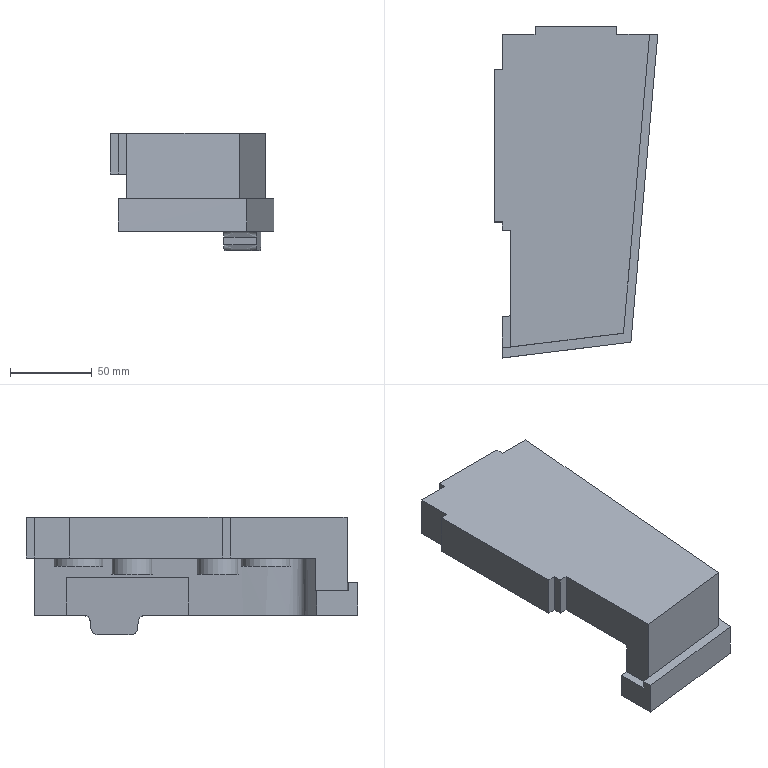Part | NX | features solid 2 | 1 solid | 41 faces | box 100.2 x 203.227 x 72 mm | volume 607434 mm3 | plane 24 | spline 13 | cylinder 4 | commonest cylinder face diameters 25 x2 30 x2